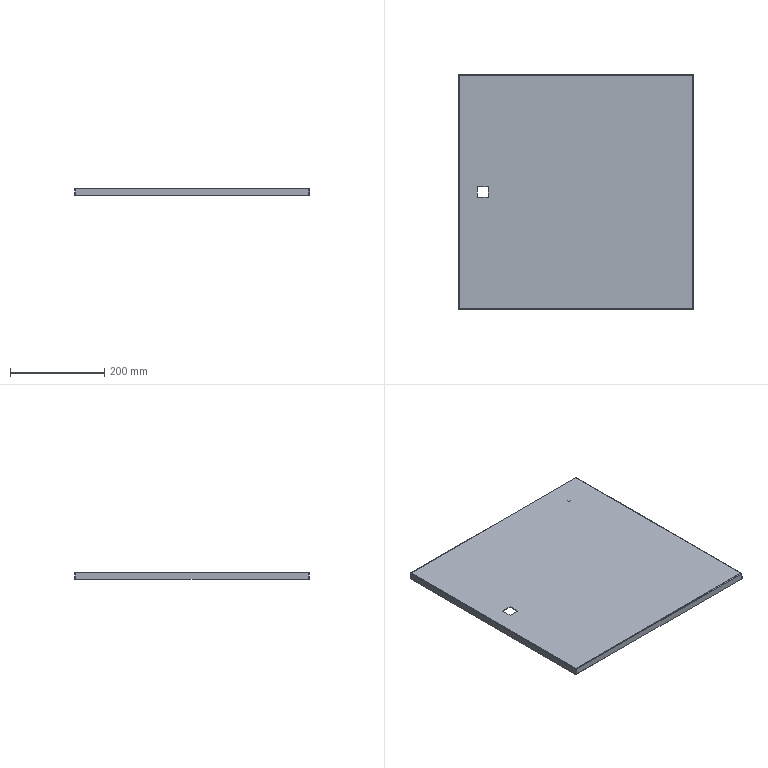Part | SolidWorks | features ICE 3, LPattern 3, EdgeFlange 2, FlatPattern 1, SMBaseFlange 1, SheetMetal 1 | 1 solid | 65 faces | box 498 x 498 x 16.5 mm | volume 410662 mm3 | plane 39 | cylinder 26 | commonest cylinder face diameters 3.2 x20 0.2 x4 6 x2